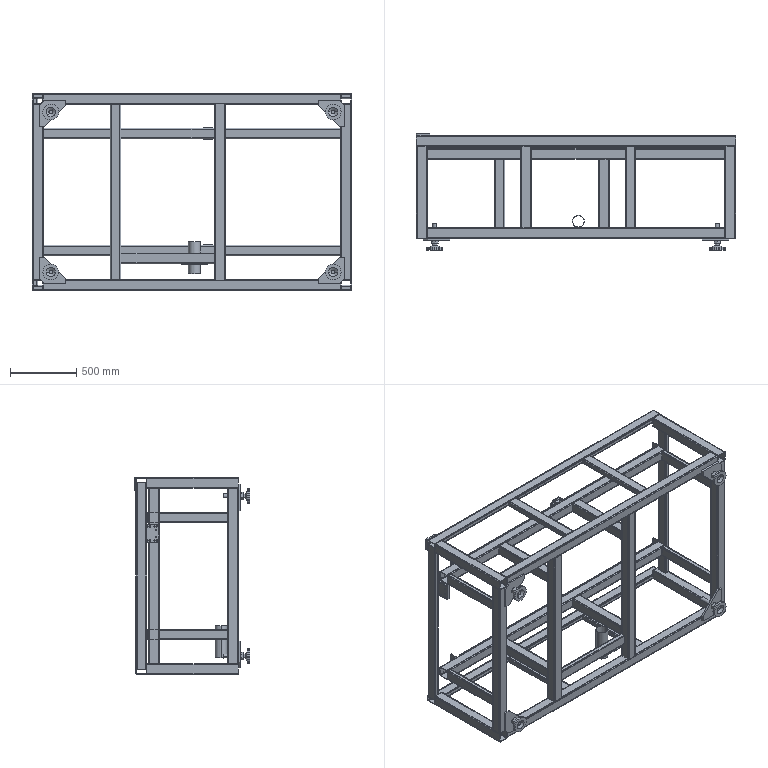Part | SolidWorks | features ReferencePattern 2, CompositeCurve 1, LocalLPattern 1 | 62 solids | 3175 faces | volume 41723102 mm3 | plane 1732 | cylinder 953 | spline 238 | cone 182 | torus 50 | sphere 20 | commonest cylinder face diameters 6.8 x208 8 x116 9 x112 16 x112 14 x108 2.822 x72